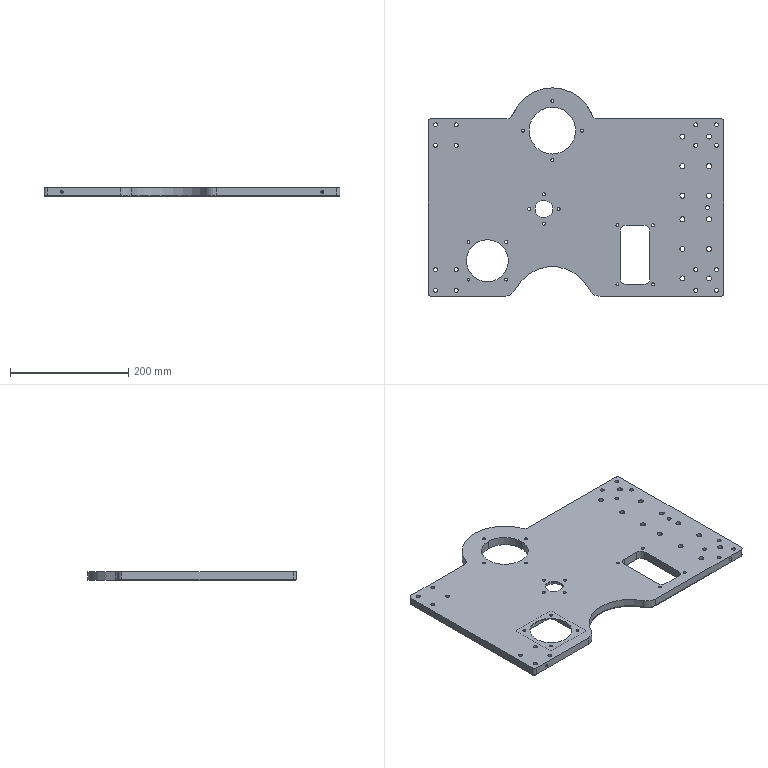NC program | Mastercam | posted with a generic post
Lines 2247 to 4160 of 11903, first 1756 of 1914 lines:
N2600 T4 M6
N2610 G0 G90 G17 G54 X-184.625 Y155.4 A0. S6000 M3
N2620 G43 H4 Z50. M8
N2630 Z1.3
N2640 G1 Z0. F600.
N2650 Y155.8 F3000.
N2660 G3 X-185.025 Y156.2 I-.4 J0.
N2670 G1 X-189.95
N2680 Y151.509
N2690 G3 X-189.55 Y151.109 I.4 J0.
N2700 G1 X-189.15
N2710 X-184.625 Y155.4
N2720 Z-.3 F600.
N2730 Y155.8 F3000.
N2740 G3 X-185.025 Y156.2 I-.4 J0.
N2750 G1 X-189.95
N2760 Y151.509
N2770 G3 X-189.55 Y151.109 I.4 J0.
N2780 G1 X-189.15
N2790 X-184.625 Y155.4
N2800 Z-.6 F600.
N2810 Y155.8 F3000.
N2820 G3 X-185.025 Y156.2 I-.4 J0.
N2830 G1 X-189.95
N2840 Y151.509
N2850 G3 X-189.55 Y151.109 I.4 J0.
N2860 G1 X-189.15
N2870 X-184.625 Y155.4
N2880 Z-.9 F600.
N2890 Y155.8 F3000.
N2900 G3 X-185.025 Y156.2 I-.4 J0.
N2910 G1 X-189.95
N2920 Y151.509
N2930 G3 X-189.55 Y151.109 I.4 J0.
N2940 G1 X-189.15
N2950 X-184.625 Y155.4
N2960 Z-1.2 F600.
N2970 Y155.8 F3000.
N2980 G3 X-185.025 Y156.2 I-.4 J0.
N2990 G1 X-189.95
N3000 Y151.509
N3010 G3 X-189.55 Y151.109 I.4 J0.
N3020 G1 X-189.15
N3030 X-184.625 Y155.4
N3040 Z-1.5 F600.
N3050 Y155.8 F3000.
N3060 G3 X-185.025 Y156.2 I-.4 J0.
N3070 G1 X-189.95
N3080 Y151.509
N3090 G3 X-189.55 Y151.109 I.4 J0.
N3100 G1 X-189.15
N3110 X-184.625 Y155.4
N3120 Z-1.8 F600.
N3130 Y155.8 F3000.
N3140 G3 X-185.025 Y156.2 I-.4 J0.
N3150 G1 X-189.95
N3160 Y151.509
N3170 G3 X-189.55 Y151.109 I.4 J0.
N3180 G1 X-189.15
N3190 X-184.625 Y155.4
N3200 Z-2.1 F600.
N3210 Y155.8 F3000.
N3220 G3 X-185.025 Y156.2 I-.4 J0.
N3230 G1 X-189.95
N3240 Y151.509
N3250 G3 X-189.55 Y151.109 I.4 J0.
N3260 G1 X-189.15
N3270 X-184.625 Y155.4
N3280 Z-2.4 F600.
N3290 Y155.8 F3000.
N3300 G3 X-185.025 Y156.2 I-.4 J0.
N3310 G1 X-189.95
N3320 Y151.509
N3330 G3 X-189.55 Y151.109 I.4 J0.
N3340 G1 X-189.15
N3350 X-184.625 Y155.4
N3360 Z-2.7 F600.
N3370 Y155.8 F3000.
N3380 G3 X-185.025 Y156.2 I-.4 J0.
N3390 G1 X-189.95
N3400 Y151.509
N3410 G3 X-189.55 Y151.109 I.4 J0.
N3420 G1 X-189.15
N3430 X-184.625 Y155.4
N3440 Z-3. F600.
N3450 Y155.8 F3000.
N3460 G3 X-185.025 Y156.2 I-.4 J0.
N3470 G1 X-189.95
N3480 Y151.509
N3490 G3 X-189.55 Y151.109 I.4 J0.
N3500 G1 X-189.15
N3510 X-184.625 Y155.4
N3520 Z-3.3 F600.
N3530 Y155.8 F3000.
N3540 G3 X-185.025 Y156.2 I-.4 J0.
N3550 G1 X-189.95
N3560 Y151.509
N3570 G3 X-189.55 Y151.109 I.4 J0.
N3580 G1 X-189.15
N3590 X-184.625 Y155.4
N3600 Z-3.6 F600.
N3610 Y155.8 F3000.
N3620 G3 X-185.025 Y156.2 I-.4 J0.
N3630 G1 X-189.95
N3640 Y151.509
N3650 G3 X-189.55 Y151.109 I.4 J0.
N3660 G1 X-189.15
N3670 X-184.625 Y155.4
N3680 Z-3.9 F600.
N3690 Y155.8 F3000.
N3700 G3 X-185.025 Y156.2 I-.4 J0.
N3710 G1 X-189.95
N3720 Y151.509
N3730 G3 X-189.55 Y151.109 I.4 J0.
N3740 G1 X-189.15
N3750 X-184.625 Y155.4
N3760 Z-4.2 F600.
N3770 Y155.8 F3000.
N3780 G3 X-185.025 Y156.2 I-.4 J0.
N3790 G1 X-189.95
N3800 Y151.509
N3810 G3 X-189.55 Y151.109 I.4 J0.
N3820 G1 X-189.15
N3830 X-184.625 Y155.4
N3840 Z-4.5 F600.
N3850 Y155.8 F3000.
N3860 G3 X-185.025 Y156.2 I-.4 J0.
N3870 G1 X-189.95
N3880 Y151.509
N3890 G3 X-189.55 Y151.109 I.4 J0.
N3900 G1 X-189.15
N3910 X-184.625 Y155.4
N3920 Z-4.8 F600.
N3930 Y155.8 F3000.
N3940 G3 X-185.025 Y156.2 I-.4 J0.
N3950 G1 X-189.95
N3960 Y151.509
N3970 G3 X-189.55 Y151.109 I.4 J0.
N3980 G1 X-189.15
N3990 X-184.625 Y155.4
N4000 Z-5.1 F600.
N4010 Y155.8 F3000.
N4020 G3 X-185.025 Y156.2 I-.4 J0.
N4030 G1 X-189.95
N4040 Y151.509
N4050 G3 X-189.55 Y151.109 I.4 J0.
N4060 G1 X-189.15
N4070 X-184.625 Y155.4
N4080 Z-5.4 F600.
N4090 Y155.8 F3000.
N4100 G3 X-185.025 Y156.2 I-.4 J0.
N4110 G1 X-189.95
N4120 Y151.509
N4130 G3 X-189.55 Y151.109 I.4 J0.
N4140 G1 X-189.15
N4150 X-184.625 Y155.4
N4160 Z-5.7 F600.
N4170 Y155.8 F3000.
N4180 G3 X-185.025 Y156.2 I-.4 J0.
N4190 G1 X-189.95
N4200 Y151.509
N4210 G3 X-189.55 Y151.109 I.4 J0.
N4220 G1 X-189.15
N4230 X-184.625 Y155.4
N4240 Z-6. F600.
N4250 Y155.8 F3000.
N4260 G3 X-185.025 Y156.2 I-.4 J0.
N4270 G1 X-189.95
N4280 Y151.509
N4290 G3 X-189.55 Y151.109 I.4 J0.
N4300 G1 X-189.15
N4310 X-184.625 Y155.4
N4320 Z-6.3 F600.
N4330 Y155.8 F3000.
N4340 G3 X-185.025 Y156.2 I-.4 J0.
N4350 G1 X-189.95
N4360 Y151.509
N4370 G3 X-189.55 Y151.109 I.4 J0.
N4380 G1 X-189.15
N4390 X-184.625 Y155.4
N4400 Z-6.6 F600.
N4410 Y155.8 F3000.
N4420 G3 X-185.025 Y156.2 I-.4 J0.
N4430 G1 X-189.95
N4440 Y151.509
N4450 G3 X-189.55 Y151.109 I.4 J0.
N4460 G1 X-189.15
N4470 X-184.625 Y155.4
N4480 Z-6.9 F600.
N4490 Y155.8 F3000.
N4500 G3 X-185.025 Y156.2 I-.4 J0.
N4510 G1 X-189.95
N4520 Y151.509
N4530 G3 X-189.55 Y151.109 I.4 J0.
N4540 G1 X-189.15
N4550 X-184.625 Y155.4
N4560 Z-7.2 F600.
N4570 Y155.8 F3000.
N4580 G3 X-185.025 Y156.2 I-.4 J0.
N4590 G1 X-189.95
N4600 Y151.509
N4610 G3 X-189.55 Y151.109 I.4 J0.
N4620 G1 X-189.15
N4630 X-184.625 Y155.4
N4640 Z-7.5 F600.
N4650 Y155.8 F3000.
N4660 G3 X-185.025 Y156.2 I-.4 J0.
N4670 G1 X-189.95
N4680 Y151.509
N4690 G3 X-189.55 Y151.109 I.4 J0.
N4700 G1 X-189.15
N4710 X-184.625 Y155.4
N4720 Z-7.8 F600.
N4730 Y155.8 F3000.
N4740 G3 X-185.025 Y156.2 I-.4 J0.
N4750 G1 X-189.95
N4760 Y151.509
N4770 G3 X-189.55 Y151.109 I.4 J0.
N4780 G1 X-189.15
N4790 X-184.625 Y155.4
N4800 Z-8.1 F600.
N4810 Y155.8 F3000.
N4820 G3 X-185.025 Y156.2 I-.4 J0.
N4830 G1 X-189.95
N4840 Y151.509
N4850 G3 X-189.55 Y151.109 I.4 J0.
N4860 G1 X-189.15
N4870 X-184.625 Y155.4
N4880 Z-8.4 F600.
N4890 Y155.8 F3000.
N4900 G3 X-185.025 Y156.2 I-.4 J0.
N4910 G1 X-189.95
N4920 Y151.509
N4930 G3 X-189.55 Y151.109 I.4 J0.
N4940 G1 X-189.15
N4950 X-184.625 Y155.4
N4960 Z-8.7 F600.
N4970 Y155.8 F3000.
N4980 G3 X-185.025 Y156.2 I-.4 J0.
N4990 G1 X-189.95
N5000 Y151.509
N5010 G3 X-189.55 Y151.109 I.4 J0.
N5020 G1 X-189.15
N5030 X-184.625 Y155.4
N5040 Z-9. F600.
N5050 Y155.8 F3000.
N5060 G3 X-185.025 Y156.2 I-.4 J0.
N5070 G1 X-189.95
N5080 Y151.509
N5090 G3 X-189.55 Y151.109 I.4 J0.
N5100 G1 X-189.15
N5110 X-184.625 Y155.4
N5120 Z-9.3 F600.
N5130 Y155.8 F3000.
N5140 G3 X-185.025 Y156.2 I-.4 J0.
N5150 G1 X-189.95
N5160 Y151.509
N5170 G3 X-189.55 Y151.109 I.4 J0.
N5180 G1 X-189.15
N5190 X-184.625 Y155.4
N5200 Z-9.6 F600.
N5210 Y155.8 F3000.
N5220 G3 X-185.025 Y156.2 I-.4 J0.
N5230 G1 X-189.95
N5240 Y151.509
N5250 G3 X-189.55 Y151.109 I.4 J0.
N5260 G1 X-189.15
N5270 X-184.625 Y155.4
N5280 Z-9.9 F600.
N5290 Y155.8 F3000.
N5300 G3 X-185.025 Y156.2 I-.4 J0.
N5310 G1 X-189.95
N5320 Y151.509
N5330 G3 X-189.55 Y151.109 I.4 J0.
N5340 G1 X-189.15
N5350 X-184.625 Y155.4
N5360 Z-10.2 F600.
N5370 Y155.8 F3000.
N5380 G3 X-185.025 Y156.2 I-.4 J0.
N5390 G1 X-189.95
N5400 Y151.509
N5410 G3 X-189.55 Y151.109 I.4 J0.
N5420 G1 X-189.15
N5430 X-184.625 Y155.4
N5440 Z-10.5 F600.
N5450 Y155.8 F3000.
N5460 G3 X-185.025 Y156.2 I-.4 J0.
N5470 G1 X-189.95
N5480 Y151.509
N5490 G3 X-189.55 Y151.109 I.4 J0.
N5500 G1 X-189.15
N5510 X-184.625 Y155.4
N5520 Z-10.8 F600.
N5530 Y155.8 F3000.
N5540 G3 X-185.025 Y156.2 I-.4 J0.
N5550 G1 X-189.95
N5560 Y151.509
N5570 G3 X-189.55 Y151.109 I.4 J0.
N5580 G1 X-189.15
N5590 X-184.625 Y155.4
N5600 Z-11.1 F600.
N5610 Y155.8 F3000.
N5620 G3 X-185.025 Y156.2 I-.4 J0.
N5630 G1 X-189.95
N5640 Y151.509
N5650 G3 X-189.55 Y151.109 I.4 J0.
N5660 G1 X-189.15
N5670 X-184.625 Y155.4
N5680 Z-11.4 F600.
N5690 Y155.8 F3000.
N5700 G3 X-185.025 Y156.2 I-.4 J0.
N5710 G1 X-189.95
N5720 Y151.509
N5730 G3 X-189.55 Y151.109 I.4 J0.
N5740 G1 X-189.15
N5750 X-184.625 Y155.4
N5760 Z-11.7 F600.
N5770 Y155.8 F3000.
N5780 G3 X-185.025 Y156.2 I-.4 J0.
N5790 G1 X-189.95
N5800 Y151.509
N5810 G3 X-189.55 Y151.109 I.4 J0.
N5820 G1 X-189.15
N5830 X-184.625 Y155.4
N5840 Z-12. F600.
N5850 Y155.8 F3000.
N5860 G3 X-185.025 Y156.2 I-.4 J0.
N5870 G1 X-189.95
N5880 Y151.509
N5890 G3 X-189.55 Y151.109 I.4 J0.
N5900 G1 X-189.15
N5910 X-184.625 Y155.4
N5920 Z-12.3 F600.
N5930 Y155.8 F3000.
N5940 G3 X-185.025 Y156.2 I-.4 J0.
N5950 G1 X-189.95
N5960 Y151.509
N5970 G3 X-189.55 Y151.109 I.4 J0.
N5980 G1 X-189.15
N5990 X-184.625 Y155.4
N6000 Z-12.6 F600.
N6010 Y155.8 F3000.
N6020 G3 X-185.025 Y156.2 I-.4 J0.
N6030 G1 X-189.95
N6040 Y151.509
N6050 G3 X-189.55 Y151.109 I.4 J0.
N6060 G1 X-189.15
N6070 X-184.625 Y155.4
N6080 Z-12.9 F600.
N6090 Y155.8 F3000.
N6100 G3 X-185.025 Y156.2 I-.4 J0.
N6110 G1 X-189.95
N6120 Y151.509
N6130 G3 X-189.55 Y151.109 I.4 J0.
N6140 G1 X-189.15
N6150 X-184.625 Y155.4
N6160 Z-13.2 F600.
N6170 Y155.8 F3000.
N6180 G3 X-185.025 Y156.2 I-.4 J0.
N6190 G1 X-189.95
N6200 Y151.509
N6210 G3 X-189.55 Y151.109 I.4 J0.
N6220 G1 X-189.15
N6230 X-184.625 Y155.4
N6240 Z-13.5 F600.
N6250 Y155.8 F3000.
N6260 G3 X-185.025 Y156.2 I-.4 J0.
N6270 G1 X-189.95
N6280 Y151.509
N6290 G3 X-189.55 Y151.109 I.4 J0.
N6300 G1 X-189.15
N6310 X-184.625 Y155.4
N6320 Z-13.8 F600.
N6330 Y155.8 F3000.
N6340 G3 X-185.025 Y156.2 I-.4 J0.
N6350 G1 X-189.95
N6360 Y151.509
N6370 G3 X-189.55 Y151.109 I.4 J0.
N6380 G1 X-189.15
N6390 G0 Z50.
N6400 Y81.2
N6410 Z1.3
N6420 G1 Z0. F600.
N6430 X-189.55 F3000.
N6440 G3 X-189.95 Y80.8 I0. J-.4
N6450 G1 Y76.3
N6460 X-185.2
N6470 G3 X-184.8 Y76.7 I0. J.4
N6480 G1 Y77.1
N6490 X-189.15 Y81.2
N6500 Z-.3 F600.
N6510 X-189.55 F3000.
N6520 G3 X-189.95 Y80.8 I0. J-.4
N6530 G1 Y76.3
N6540 X-185.2
N6550 G3 X-184.8 Y76.7 I0. J.4
N6560 G1 Y77.1
N6570 X-189.15 Y81.2
N6580 Z-.6 F600.
N6590 X-189.55 F3000.
N6600 G3 X-189.95 Y80.8 I0. J-.4
N6610 G1 Y76.3
N6620 X-185.2
N6630 G3 X-184.8 Y76.7 I0. J.4
N6640 G1 Y77.1
N6650 X-189.15 Y81.2
N6660 Z-.9 F600.
N6670 X-189.55 F3000.
N6680 G3 X-189.95 Y80.8 I0. J-.4
N6690 G1 Y76.3
N6700 X-185.2
N6710 G3 X-184.8 Y76.7 I0. J.4
N6720 G1 Y77.1
N6730 X-189.15 Y81.2
N6740 Z-1.2 F600.
N6750 X-189.55 F3000.
N6760 G3 X-189.95 Y80.8 I0. J-.4
N6770 G1 Y76.3
N6780 X-185.2
N6790 G3 X-184.8 Y76.7 I0. J.4
N6800 G1 Y77.1
N6810 X-189.15 Y81.2
N6820 Z-1.5 F600.
N6830 X-189.55 F3000.
N6840 G3 X-189.95 Y80.8 I0. J-.4
N6850 G1 Y76.3
N6860 X-185.2
N6870 G3 X-184.8 Y76.7 I0. J.4
N6880 G1 Y77.1
N6890 X-189.15 Y81.2
N6900 Z-1.8 F600.
N6910 X-189.55 F3000.
N6920 G3 X-189.95 Y80.8 I0. J-.4
N6930 G1 Y76.3
N6940 X-185.2
N6950 G3 X-184.8 Y76.7 I0. J.4
N6960 G1 Y77.1
N6970 X-189.15 Y81.2
N6980 Z-2.1 F600.
N6990 X-189.55 F3000.
N7000 G3 X-189.95 Y80.8 I0. J-.4
N7010 G1 Y76.3
N7020 X-185.2
N7030 G3 X-184.8 Y76.7 I0. J.4
N7040 G1 Y77.1
N7050 X-189.15 Y81.2
N7060 Z-2.4 F600.
N7070 X-189.55 F3000.
N7080 G3 X-189.95 Y80.8 I0. J-.4
N7090 G1 Y76.3
N7100 X-185.2
N7110 G3 X-184.8 Y76.7 I0. J.4
N7120 G1 Y77.1
N7130 X-189.15 Y81.2
N7140 Z-2.7 F600.
N7150 X-189.55 F3000.
N7160 G3 X-189.95 Y80.8 I0. J-.4
N7170 G1 Y76.3
N7180 X-185.2
N7190 G3 X-184.8 Y76.7 I0. J.4
N7200 G1 Y77.1
N7210 X-189.15 Y81.2
N7220 Z-3. F600.
N7230 X-189.55 F3000.
N7240 G3 X-189.95 Y80.8 I0. J-.4
N7250 G1 Y76.3
N7260 X-185.2
N7270 G3 X-184.8 Y76.7 I0. J.4
N7280 G1 Y77.1
N7290 X-189.15 Y81.2
N7300 Z-3.3 F600.
N7310 X-189.55 F3000.
N7320 G3 X-189.95 Y80.8 I0. J-.4
N7330 G1 Y76.3
N7340 X-185.2
N7350 G3 X-184.8 Y76.7 I0. J.4
N7360 G1 Y77.1
N7370 X-189.15 Y81.2
N7380 Z-3.6 F600.
N7390 X-189.55 F3000.
N7400 G3 X-189.95 Y80.8 I0. J-.4
N7410 G1 Y76.3
N7420 X-185.2
N7430 G3 X-184.8 Y76.7 I0. J.4
N7440 G1 Y77.1
N7450 X-189.15 Y81.2
N7460 Z-3.9 F600.
N7470 X-189.55 F3000.
N7480 G3 X-189.95 Y80.8 I0. J-.4
N7490 G1 Y76.3
N7500 X-185.2
N7510 G3 X-184.8 Y76.7 I0. J.4
N7520 G1 Y77.1
N7530 X-189.15 Y81.2
N7540 Z-4.2 F600.
N7550 X-189.55 F3000.
N7560 G3 X-189.95 Y80.8 I0. J-.4
N7570 G1 Y76.3
N7580 X-185.2
N7590 G3 X-184.8 Y76.7 I0. J.4
N7600 G1 Y77.1
N7610 X-189.15 Y81.2
N7620 Z-4.5 F600.
N7630 X-189.55 F3000.
N7640 G3 X-189.95 Y80.8 I0. J-.4
N7650 G1 Y76.3
N7660 X-185.2
N7670 G3 X-184.8 Y76.7 I0. J.4
N7680 G1 Y77.1
N7690 X-189.15 Y81.2
N7700 Z-4.8 F600.
N7710 X-189.55 F3000.
N7720 G3 X-189.95 Y80.8 I0. J-.4
N7730 G1 Y76.3
N7740 X-185.2
N7750 G3 X-184.8 Y76.7 I0. J.4
N7760 G1 Y77.1
N7770 X-189.15 Y81.2
N7780 Z-5.1 F600.
N7790 X-189.55 F3000.
N7800 G3 X-189.95 Y80.8 I0. J-.4
N7810 G1 Y76.3
N7820 X-185.2
N7830 G3 X-184.8 Y76.7 I0. J.4
N7840 G1 Y77.1
N7850 X-189.15 Y81.2
N7860 Z-5.4 F600.
N7870 X-189.55 F3000.
N7880 G3 X-189.95 Y80.8 I0. J-.4
N7890 G1 Y76.3
N7900 X-185.2
N7910 G3 X-184.8 Y76.7 I0. J.4
N7920 G1 Y77.1
N7930 X-189.15 Y81.2
N7940 Z-5.7 F600.
N7950 X-189.55 F3000.
N7960 G3 X-189.95 Y80.8 I0. J-.4
N7970 G1 Y76.3
N7980 X-185.2
N7990 G3 X-184.8 Y76.7 I0. J.4
N8000 G1 Y77.1
N8010 X-189.15 Y81.2
N8020 Z-6. F600.
N8030 X-189.55 F3000.
N8040 G3 X-189.95 Y80.8 I0. J-.4
N8050 G1 Y76.3
N8060 X-185.2
N8070 G3 X-184.8 Y76.7 I0. J.4
N8080 G1 Y77.1
N8090 X-189.15 Y81.2
N8100 Z-6.3 F600.
N8110 X-189.55 F3000.
N8120 G3 X-189.95 Y80.8 I0. J-.4
N8130 G1 Y76.3
N8140 X-185.2
N8150 G3 X-184.8 Y76.7 I0. J.4
N8160 G1 Y77.1
N8170 X-189.15 Y81.2
N8180 Z-6.6 F600.
N8190 X-189.55 F3000.
N8200 G3 X-189.95 Y80.8 I0. J-.4
N8210 G1 Y76.3
N8220 X-185.2
N8230 G3 X-184.8 Y76.7 I0. J.4
N8240 G1 Y77.1
N8250 X-189.15 Y81.2
N8260 Z-6.9 F600.
N8270 X-189.55 F3000.
N8280 G3 X-189.95 Y80.8 I0. J-.4
N8290 G1 Y76.3
N8300 X-185.2
N8310 G3 X-184.8 Y76.7 I0. J.4
N8320 G1 Y77.1
N8330 X-189.15 Y81.2
N8340 Z-7.2 F600.
N8350 X-189.55 F3000.
N8360 G3 X-189.95 Y80.8 I0. J-.4
N8370 G1 Y76.3
N8380 X-185.2
N8390 G3 X-184.8 Y76.7 I0. J.4
N8400 G1 Y77.1
N8410 X-189.15 Y81.2
N8420 Z-7.5 F600.
N8430 X-189.55 F3000.
N8440 G3 X-189.95 Y80.8 I0. J-.4
N8450 G1 Y76.3
N8460 X-185.2
N8470 G3 X-184.8 Y76.7 I0. J.4
N8480 G1 Y77.1
N8490 X-189.15 Y81.2
N8500 Z-7.8 F600.
N8510 X-189.55 F3000.
N8520 G3 X-189.95 Y80.8 I0. J-.4
N8530 G1 Y76.3
N8540 X-185.2
N8550 G3 X-184.8 Y76.7 I0. J.4
N8560 G1 Y77.1
N8570 X-189.15 Y81.2
N8580 Z-8.1 F600.
N8590 X-189.55 F3000.
N8600 G3 X-189.95 Y80.8 I0. J-.4
N8610 G1 Y76.3
N8620 X-185.2
N8630 G3 X-184.8 Y76.7 I0. J.4
N8640 G1 Y77.1
N8650 X-189.15 Y81.2
N8660 Z-8.4 F600.
N8670 X-189.55 F3000.
N8680 G3 X-189.95 Y80.8 I0. J-.4
N8690 G1 Y76.3
N8700 X-185.2
N8710 G3 X-184.8 Y76.7 I0. J.4
N8720 G1 Y77.1
N8730 X-189.15 Y81.2
N8740 Z-8.7 F600.
N8750 X-189.55 F3000.
N8760 G3 X-189.95 Y80.8 I0. J-.4
N8770 G1 Y76.3
N8780 X-185.2
N8790 G3 X-184.8 Y76.7 I0. J.4
N8800 G1 Y77.1
N8810 X-189.15 Y81.2
N8820 Z-9. F600.
N8830 X-189.55 F3000.
N8840 G3 X-189.95 Y80.8 I0. J-.4
N8850 G1 Y76.3
N8860 X-185.2
N8870 G3 X-184.8 Y76.7 I0. J.4
N8880 G1 Y77.1
N8890 X-189.15 Y81.2
N8900 Z-9.3 F600.
N8910 X-189.55 F3000.
N8920 G3 X-189.95 Y80.8 I0. J-.4
N8930 G1 Y76.3
N8940 X-185.2
N8950 G3 X-184.8 Y76.7 I0. J.4
N8960 G1 Y77.1
N8970 X-189.15 Y81.2
N8980 Z-9.6 F600.
N8990 X-189.55 F3000.
N9000 G3 X-189.95 Y80.8 I0. J-.4
N9010 G1 Y76.3
N9020 X-185.2
N9030 G3 X-184.8 Y76.7 I0. J.4
N9040 G1 Y77.1
N9050 X-189.15 Y81.2
N9060 Z-9.9 F600.
N9070 X-189.55 F3000.
N9080 G3 X-189.95 Y80.8 I0. J-.4
N9090 G1 Y76.3
N9100 X-185.2
N9110 G3 X-184.8 Y76.7 I0. J.4
N9120 G1 Y77.1
N9130 X-189.15 Y81.2
N9140 Z-10.2 F600.
N9150 X-189.55 F3000.
N9160 G3 X-189.95 Y80.8 I0. J-.4
N9170 G1 Y76.3
N9180 X-185.2
N9190 G3 X-184.8 Y76.7 I0. J.4
N9200 G1 Y77.1
N9210 X-189.15 Y81.2
N9220 Z-10.5 F600.
N9230 X-189.55 F3000.
N9240 G3 X-189.95 Y80.8 I0. J-.4
N9250 G1 Y76.3
N9260 X-185.2
N9270 G3 X-184.8 Y76.7 I0. J.4
N9280 G1 Y77.1
N9290 X-189.15 Y81.2
N9300 Z-10.8 F600.
N9310 X-189.55 F3000.
N9320 G3 X-189.95 Y80.8 I0. J-.4
N9330 G1 Y76.3
N9340 X-185.2
N9350 G3 X-184.8 Y76.7 I0. J.4
N9360 G1 Y77.1
N9370 X-189.15 Y81.2
N9380 Z-11.1 F600.
N9390 X-189.55 F3000.
N9400 G3 X-189.95 Y80.8 I0. J-.4
N9410 G1 Y76.3
N9420 X-185.2
N9430 G3 X-184.8 Y76.7 I0. J.4
N9440 G1 Y77.1
N9450 X-189.15 Y81.2
N9460 Z-11.4 F600.
N9470 X-189.55 F3000.
N9480 G3 X-189.95 Y80.8 I0. J-.4
N9490 G1 Y76.3
N9500 X-185.2
N9510 G3 X-184.8 Y76.7 I0. J.4
N9520 G1 Y77.1
N9530 X-189.15 Y81.2
N9540 Z-11.7 F600.
N9550 X-189.55 F3000.
N9560 G3 X-189.95 Y80.8 I0. J-.4
N9570 G1 Y76.3
N9580 X-185.2
N9590 G3 X-184.8 Y76.7 I0. J.4
N9600 G1 Y77.1
N9610 X-189.15 Y81.2
N9620 Z-12. F600.
N9630 X-189.55 F3000.
N9640 G3 X-189.95 Y80.8 I0. J-.4
N9650 G1 Y76.3
N9660 X-185.2
N9670 G3 X-184.8 Y76.7 I0. J.4
N9680 G1 Y77.1
N9690 X-189.15 Y81.2
N9700 Z-12.3 F600.
N9710 X-189.55 F3000.
N9720 G3 X-189.95 Y80.8 I0. J-.4
N9730 G1 Y76.3
N9740 X-185.2
N9750 G3 X-184.8 Y76.7 I0. J.4
N9760 G1 Y77.1
N9770 X-189.15 Y81.2
N9780 Z-12.6 F600.
N9790 X-189.55 F3000.
N9800 G3 X-189.95 Y80.8 I0. J-.4
N9810 G1 Y76.3
N9820 X-185.2
N9830 G3 X-184.8 Y76.7 I0. J.4
N9840 G1 Y77.1
N9850 X-189.15 Y81.2
N9860 Z-12.9 F600.
N9870 X-189.55 F3000.
N9880 G3 X-189.95 Y80.8 I0. J-.4
N9890 G1 Y76.3
N9900 X-185.2
N9910 G3 X-184.8 Y76.7 I0. J.4
N9920 G1 Y77.1
N9930 X-189.15 Y81.2
N9940 Z-13.2 F600.
N9950 X-189.55 F3000.
N9960 G3 X-189.95 Y80.8 I0. J-.4
N9970 G1 Y76.3
N9980 X-185.2
N9990 G3 X-184.8 Y76.7 I0. J.4
N100 G1 Y77.1
N110 X-189.15 Y81.2
N120 Z-13.5 F600.
N130 X-189.55 F3000.
N140 G3 X-189.95 Y80.8 I0. J-.4
N150 G1 Y76.3
N160 X-185.2
N170 G3 X-184.8 Y76.7 I0. J.4
N180 G1 Y77.1
N190 X-189.15 Y81.2
N200 Z-13.8 F600.
N210 X-189.55 F3000.
N220 G3 X-189.95 Y80.8 I0. J-.4
N230 G1 Y76.3
N240 X-185.2
N250 G3 X-184.8 Y76.7 I0. J.4
N260 G1 Y77.1
N270 G0 Z50.
N280 X-115.2
N290 Z1.3
N300 G1 Z0. F600.
N310 Y76.7 F3000.
N320 G3 X-114.8 Y76.3 I.4 J0.
N330 G1 X-110.05
N340 Y80.882
N350 G3 X-110.45 Y81.282 I-.4 J0.
N360 G1 X-110.85
N370 X-115.2 Y77.1
N380 Z-.3 F600.
N390 Y76.7 F3000.
N400 G3 X-114.8 Y76.3 I.4 J0.
N410 G1 X-110.05
N420 Y80.882
N430 G3 X-110.45 Y81.282 I-.4 J0.
N440 G1 X-110.85
N450 X-115.2 Y77.1
N460 Z-.6 F600.
N470 Y76.7 F3000.
N480 G3 X-114.8 Y76.3 I.4 J0.
N490 G1 X-110.05
N500 Y80.882
N510 G3 X-110.45 Y81.282 I-.4 J0.
N520 G1 X-110.85
N530 X-115.2 Y77.1
N540 Z-.9 F600.
N550 Y76.7 F3000.
N560 G3 X-114.8 Y76.3 I.4 J0.
N570 G1 X-110.05
N580 Y80.882
N590 G3 X-110.45 Y81.282 I-.4 J0.
N600 G1 X-110.85
N610 X-115.2 Y77.1
N620 Z-1.2 F600.
N630 Y76.7 F3000.
N640 G3 X-114.8 Y76.3 I.4 J0.
N650 G1 X-110.05
N660 Y80.882
N670 G3 X-110.45 Y81.282 I-.4 J0.
N680 G1 X-110.85
N690 X-115.2 Y77.1
N700 Z-1.5 F600.
N710 Y76.7 F3000.
N720 G3 X-114.8 Y76.3 I.4 J0.
N730 G1 X-110.05
N740 Y80.882
N750 G3 X-110.45 Y81.282 I-.4 J0.
N760 G1 X-110.85
N770 X-115.2 Y77.1
N780 Z-1.8 F600.
N790 Y76.7 F3000.
N800 G3 X-114.8 Y76.3 I.4 J0.
N810 G1 X-110.05
N820 Y80.882
N830 G3 X-110.45 Y81.282 I-.4 J0.
N840 G1 X-110.85
N850 X-115.2 Y77.1
N860 Z-2.1 F600.
N870 Y76.7 F3000.
N880 G3 X-114.8 Y76.3 I.4 J0.
N890 G1 X-110.05
N900 Y80.882
N910 G3 X-110.45 Y81.282 I-.4 J0.
N920 G1 X-110.85
N930 X-115.2 Y77.1
N940 Z-2.4 F600.
N950 Y76.7 F3000.
N960 G3 X-114.8 Y76.3 I.4 J0.
N970 G1 X-110.05
N980 Y80.882
N990 G3 X-110.45 Y81.282 I-.4 J0.
N1000 G1 X-110.85
N1010 X-115.2 Y77.1
N1020 Z-2.7 F600.
N1030 Y76.7 F3000.
N1040 G3 X-114.8 Y76.3 I.4 J0.
N1050 G1 X-110.05
N1060 Y80.882
N1070 G3 X-110.45 Y81.282 I-.4 J0.
N1080 G1 X-110.85
N1090 X-115.2 Y77.1
N1100 Z-3. F600.
N1110 Y76.7 F3000.
N1120 G3 X-114.8 Y76.3 I.4 J0.
N1130 G1 X-110.05
N1140 Y80.882
N1150 G3 X-110.45 Y81.282 I-.4 J0.
N1160 G1 X-110.85
N1170 X-115.2 Y77.1
N1180 Z-3.3 F600.
N1190 Y76.7 F3000.
N1200 G3 X-114.8 Y76.3 I.4 J0.
N1210 G1 X-110.05
N1220 Y80.882
N1230 G3 X-110.45 Y81.282 I-.4 J0.
N1240 G1 X-110.85
N1250 X-115.2 Y77.1
N1260 Z-3.6 F600.
N1270 Y76.7 F3000.
N1280 G3 X-114.8 Y76.3 I.4 J0.
N1290 G1 X-110.05
N1300 Y80.882
N1310 G3 X-110.45 Y81.282 I-.4 J0.
N1320 G1 X-110.85
N1330 X-115.2 Y77.1
N1340 Z-3.9 F600.
N1350 Y76.7 F3000.
N1360 G3 X-114.8 Y76.3 I.4 J0.
N1370 G1 X-110.05
N1380 Y80.882
N1390 G3 X-110.45 Y81.282 I-.4 J0.
N1400 G1 X-110.85
N1410 X-115.2 Y77.1
N1420 Z-4.2 F600.
N1430 Y76.7 F3000.
N1440 G3 X-114.8 Y76.3 I.4 J0.
N1450 G1 X-110.05
N1460 Y80.882
N1470 G3 X-110.45 Y81.282 I-.4 J0.
N1480 G1 X-110.85
N1490 X-115.2 Y77.1
N1500 Z-4.5 F600.
N1510 Y76.7 F3000.
N1520 G3 X-114.8 Y76.3 I.4 J0.
N1530 G1 X-110.05
N1540 Y80.882
N1550 G3 X-110.45 Y81.282 I-.4 J0.
N1560 G1 X-110.85
N1570 X-115.2 Y77.1
N1580 Z-4.8 F600.
N1590 Y76.7 F3000.
N1600 G3 X-114.8 Y76.3 I.4 J0.
N1610 G1 X-110.05
N1620 Y80.882
N1630 G3 X-110.45 Y81.282 I-.4 J0.
N1640 G1 X-110.85
N1650 X-115.2 Y77.1
N1660 Z-5.1 F600.
N1670 Y76.7 F3000.
N1680 G3 X-114.8 Y76.3 I.4 J0.
N1690 G1 X-110.05
N1700 Y80.882
N1710 G3 X-110.45 Y81.282 I-.4 J0.
N1720 G1 X-110.85
N1730 X-115.2 Y77.1
N1740 Z-5.4 F600.
N1750 Y76.7 F3000.
N1760 G3 X-114.8 Y76.3 I.4 J0.
N1770 G1 X-110.05
N1780 Y80.882
N1790 G3 X-110.45 Y81.282 I-.4 J0.
N1800 G1 X-110.85
N1810 X-115.2 Y77.1
N1820 Z-5.7 F600.
N1830 Y76.7 F3000.
N1840 G3 X-114.8 Y76.3 I.4 J0.
N1850 G1 X-110.05
N1860 Y80.882
N1870 G3 X-110.45 Y81.282 I-.4 J0.
N1880 G1 X-110.85
N1890 X-115.2 Y77.1
N1900 Z-6. F600.
N1910 Y76.7 F3000.
N1920 G3 X-114.8 Y76.3 I.4 J0.
N1930 G1 X-110.05
N1940 Y80.882
N1950 G3 X-110.45 Y81.282 I-.4 J0.
N1960 G1 X-110.85
N1970 X-115.2 Y77.1
N1980 Z-6.3 F600.
N1990 Y76.7 F3000.
N2000 G3 X-114.8 Y76.3 I.4 J0.
N2010 G1 X-110.05
N2020 Y80.882
N2030 G3 X-110.45 Y81.282 I-.4 J0.
N2040 G1 X-110.85
N2050 X-115.2 Y77.1
N2060 Z-6.6 F600.
N2070 Y76.7 F3000.
N2080 G3 X-114.8 Y76.3 I.4 J0.
N2090 G1 X-110.05
N2100 Y80.882
N2110 G3 X-110.45 Y81.282 I-.4 J0.
N2120 G1 X-110.85
N2130 X-115.2 Y77.1
N2140 Z-6.9 F600.
N2150 Y76.7 F3000.
N2160 G3 X-114.8 Y76.3 I.4 J0.
N2170 G1 X-110.05
N2180 Y80.882
N2190 G3 X-110.45 Y81.282 I-.4 J0.
N2200 G1 X-110.85
N2210 X-115.2 Y77.1
N2220 Z-7.2 F600.
N2230 Y76.7 F3000.
N2240 G3 X-114.8 Y76.3 I.4 J0.
N2250 G1 X-110.05
N2260 Y80.882
N2270 G3 X-110.45 Y81.282 I-.4 J0.
N2280 G1 X-110.85
N2290 X-115.2 Y77.1
N2300 Z-7.5 F600.
N2310 Y76.7 F3000.
N2320 G3 X-114.8 Y76.3 I.4 J0.
N2330 G1 X-110.05
N2340 Y80.882
N2350 G3 X-110.45 Y81.282 I-.4 J0.
N2360 G1 X-110.85
N2370 X-115.2 Y77.1
N2380 Z-7.8 F600.
N2390 Y76.7 F3000.
N2400 G3 X-114.8 Y76.3 I.4 J0.
N2410 G1 X-110.05
N2420 Y80.882
N2430 G3 X-110.45 Y81.282 I-.4 J0.
N2440 G1 X-110.85
N2450 X-115.2 Y77.1
N2460 Z-8.1 F600.
N2470 Y76.7 F3000.
N2480 G3 X-114.8 Y76.3 I.4 J0.
N2490 G1 X-110.05
N2500 Y80.882
N2510 G3 X-110.45 Y81.282 I-.4 J0.
N2520 G1 X-110.85
N2530 X-115.2 Y77.1
N2540 Z-8.4 F600.
N2550 Y76.7 F3000.
N2560 G3 X-114.8 Y76.3 I.4 J0.
N2570 G1 X-110.05
N2580 Y80.882
N2590 G3 X-110.45 Y81.282 I-.4 J0.
N2600 G1 X-110.85
N2610 X-115.2 Y77.1
N2620 Z-8.7 F600.
N2630 Y76.7 F3000.
N2640 G3 X-114.8 Y76.3 I.4 J0.
N2650 G1 X-110.05
N2660 Y80.882
N2670 G3 X-110.45 Y81.282 I-.4 J0.
N2680 G1 X-110.85
N2690 X-115.2 Y77.1
N2700 Z-9. F600.
N2710 Y76.7 F3000.
N2720 G3 X-114.8 Y76.3 I.4 J0.
N2730 G1 X-110.05
N2740 Y80.882
N2750 G3 X-110.45 Y81.282 I-.4 J0.
N2760 G1 X-110.85
N2770 X-115.2 Y77.1
N2780 Z-9.3 F600.
N2790 Y76.7 F3000.
N2800 G3 X-114.8 Y76.3 I.4 J0.
N2810 G1 X-110.05
N2820 Y80.882
N2830 G3 X-110.45 Y81.282 I-.4 J0.
N2840 G1 X-110.85
N2850 X-115.2 Y77.1
N2860 Z-9.6 F600.
N2870 Y76.7 F3000.
N2880 G3 X-114.8 Y76.3 I.4 J0.
N2890 G1 X-110.05
N2900 Y80.882
N2910 G3 X-110.45 Y81.282 I-.4 J0.
N2920 G1 X-110.85
N2930 X-115.2 Y77.1
N2940 Z-9.9 F600.
N2950 Y76.7 F3000.
N2960 G3 X-114.8 Y76.3 I.4 J0.
N2970 G1 X-110.05
N2980 Y80.882
N2990 G3 X-110.45 Y81.282 I-.4 J0.
N3000 G1 X-110.85
N3010 X-115.2 Y77.1
N3020 Z-10.2 F600.
N3030 Y76.7 F3000.
N3040 G3 X-114.8 Y76.3 I.4 J0.
N3050 G1 X-110.05
N3060 Y80.882
N3070 G3 X-110.45 Y81.282 I-.4 J0.
N3080 G1 X-110.85
N3090 X-115.2 Y77.1
N3100 Z-10.5 F600.
N3110 Y76.7 F3000.
N3120 G3 X-114.8 Y76.3 I.4 J0.
N3130 G1 X-110.05
N3140 Y80.882
N3150 G3 X-110.45 Y81.282 I-.4 J0.
N3160 G1 X-110.85
N3170 X-115.2 Y77.1
N3180 Z-10.8 F600.
N3190 Y76.7 F3000.
N3200 G3 X-114.8 Y76.3 I.4 J0.
N3210 G1 X-110.05
N3220 Y80.882
N3230 G3 X-110.45 Y81.282 I-.4 J0.
N3240 G1 X-110.85
N3250 X-115.2 Y77.1
N3260 Z-11.1 F600.
N3270 Y76.7 F3000.
N3280 G3 X-114.8 Y76.3 I.4 J0.
N3290 G1 X-110.05
N3300 Y80.882
N3310 G3 X-110.45 Y81.282 I-.4 J0.
N3320 G1 X-110.85
N3330 X-115.2 Y77.1
N3340 Z-11.4 F600.
N3350 Y76.7 F3000.
N3360 G3 X-114.8 Y76.3 I.4 J0.
N3370 G1 X-110.05
N3380 Y80.882
N3390 G3 X-110.45 Y81.282 I-.4 J0.
N3400 G1 X-110.85
N3410 X-115.2 Y77.1
N3420 Z-11.7 F600.
N3430 Y76.7 F3000.
N3440 G3 X-114.8 Y76.3 I.4 J0.
N3450 G1 X-110.05
N3460 Y80.882
N3470 G3 X-110.45 Y81.282 I-.4 J0.
N3480 G1 X-110.85
N3490 X-115.2 Y77.1
N3500 Z-12. F600.
N3510 Y76.7 F3000.
N3520 G3 X-114.8 Y76.3 I.4 J0.
N3530 G1 X-110.05
N3540 Y80.882
N3550 G3 X-110.45 Y81.282 I-.4 J0.
N3560 G1 X-110.85
N3570 X-115.2 Y77.1
N3580 Z-12.3 F600.
N3590 Y76.7 F3000.
N3600 G3 X-114.8 Y76.3 I.4 J0.
N3610 G1 X-110.05
N3620 Y80.882
N3630 G3 X-110.45 Y81.282 I-.4 J0.
N3640 G1 X-110.85
N3650 X-115.2 Y77.1
N3660 Z-12.6 F600.
N3670 Y76.7 F3000.
N3680 G3 X-114.8 Y76.3 I.4 J0.
N3690 G1 X-110.05
N3700 Y80.882
N3710 G3 X-110.45 Y81.282 I-.4 J0.
N3720 G1 X-110.85
N3730 X-115.2 Y77.1
N3740 Z-12.9 F600.
N3750 Y76.7 F3000.
N3760 G3 X-114.8 Y76.3 I.4 J0.
N3770 G1 X-110.05
N3780 Y80.882
N3790 G3 X-110.45 Y81.282 I-.4 J0.
N3800 G1 X-110.85
N3810 X-115.2 Y77.1
N3820 Z-13.2 F600.
N3830 Y76.7 F3000.
N3840 G3 X-114.8 Y76.3 I.4 J0.
N3850 G1 X-110.05
N3860 Y80.882
N3870 G3 X-110.45 Y81.282 I-.4 J0.
N3880 G1 X-110.85
N3890 X-115.2 Y77.1
N3900 Z-13.5 F600.
N3910 Y76.7 F3000.
N3920 G3 X-114.8 Y76.3 I.4 J0.
N3930 G1 X-110.05
N3940 Y80.882
N3950 G3 X-110.45 Y81.282 I-.4 J0.
N3960 G1 X-110.85
N3970 X-115.2 Y77.1
N3980 Z-13.8 F600.
N3990 Y76.7 F3000.
N4000 G3 X-114.8 Y76.3 I.4 J0.
N4010 G1 X-110.05
N4020 Y80.882
N4030 G3 X-110.45 Y81.282 I-.4 J0.
N4040 G1 X-110.85
N4050 G0 Z50.
N4060 Y151.185
N4070 Z1.3
N4080 G1 Z0. F600.
N4090 X-110.45 F3000.
N4100 G3 X-110.05 Y151.585 I0. J.4
N4110 G1 Y156.2
N4120 X-115.015
N4130 G3 X-115.415 Y155.8 I0. J-.4
N4140 G1 Y155.4
N4150 X-110.85 Y151.185
N4160 Z-.3 F600.
N4170 X-110.45 F3000.
N4180 G3 X-110.05 Y151.585 I0. J.4
N4190 G1 Y156.2
N4200 X-115.015
N4210 G3 X-115.415 Y155.8 I0. J-.4
N4220 G1 Y155.4
N4230 X-110.85 Y151.185
N4240 Z-.6 F600.
N4250 X-110.45 F3000.
N4260 G3 X-110.05 Y151.585 I0. J.4
N4270 G1 Y156.2
N4280 X-115.015
N4290 G3 X-115.415 Y155.8 I0. J-.4
N4300 G1 Y155.4
N4310 X-110.85 Y151.185
N4320 Z-.9 F600.
N4330 X-110.45 F3000.
N4340 G3 X-110.05 Y151.585 I0. J.4
N4350 G1 Y156.2
N4360 X-115.015
N4370 G3 X-115.415 Y155.8 I0. J-.4
N4380 G1 Y155.4
N4390 X-110.85 Y151.185
N4400 Z-1.2 F600.
N4410 X-110.45 F3000.
N4420 G3 X-110.05 Y151.585 I0. J.4
N4430 G1 Y156.2
N4440 X-115.015
N4450 G3 X-115.415 Y155.8 I0. J-.4
N4460 G1 Y155.4
N4470 X-110.85 Y151.185
N4480 Z-1.5 F600.
N4490 X-110.45 F3000.
N4500 G3 X-110.05 Y151.585 I0. J.4
N4510 G1 Y156.2
N4520 X-115.015
N4530 G3 X-115.415 Y155.8 I0. J-.4
N4540 G1 Y155.4
N4550 X-110.85 Y151.185
N4560 Z-1.8 F600.
N4570 X-110.45 F3000.
N4580 G3 X-110.05 Y151.585 I0. J.4
N4590 G1 Y156.2
N4600 X-115.015
N4610 G3 X-115.415 Y155.8 I0. J-.4
N4620 G1 Y155.4
N4630 X-110.85 Y151.185
N4640 Z-2.1 F600.
N4650 X-110.45 F3000.
N4660 G3 X-110.05 Y151.585 I0. J.4
N4670 G1 Y156.2
N4680 X-115.015
N4690 G3 X-115.415 Y155.8 I0. J-.4
N4700 G1 Y155.4
N4710 X-110.85 Y151.185
N4720 Z-2.4 F600.
N4730 X-110.45 F3000.
N4740 G3 X-110.05 Y151.585 I0. J.4
N4750 G1 Y156.2
N4760 X-115.015
N4770 G3 X-115.415 Y155.8 I0. J-.4
N4780 G1 Y155.4
N4790 X-110.85 Y151.185
N4800 Z-2.7 F600.
N4810 X-110.45 F3000.
N4820 G3 X-110.05 Y151.585 I0. J.4
N4830 G1 Y156.2
N4840 X-115.015
N4850 G3 X-115.415 Y155.8 I0. J-.4
N4860 G1 Y155.4
N4870 X-110.85 Y151.185
N4880 Z-3. F600.
N4890 X-110.45 F3000.
N4900 G3 X-110.05 Y151.585 I0. J.4
N4910 G1 Y156.2
N4920 X-115.015
N4930 G3 X-115.415 Y155.8 I0. J-.4
N4940 G1 Y155.4
N4950 X-110.85 Y151.185
N4960 Z-3.3 F600.
N4970 X-110.45 F3000.
N4980 G3 X-110.05 Y151.585 I0. J.4
N4990 G1 Y156.2
N5000 X-115.015
N5010 G3 X-115.415 Y155.8 I0. J-.4
N5020 G1 Y155.4
N5030 X-110.85 Y151.185
N5040 Z-3.6 F600.
N5050 X-110.45 F3000.
N5060 G3 X-110.05 Y151.585 I0. J.4
N5070 G1 Y156.2
N5080 X-115.015
N5090 G3 X-115.415 Y155.8 I0. J-.4
N5100 G1 Y155.4
N5110 X-110.85 Y151.185
N5120 Z-3.9 F600.
N5130 X-110.45 F3000.
N5140 G3 X-110.05 Y151.585 I0. J.4
N5150 G1 Y156.2
N5160 X-115.015
N5170 G3 X-115.415 Y155.8 I0. J-.4
N5180 G1 Y155.4
N5190 X-110.85 Y151.185
N5200 Z-4.2 F600.
N5210 X-110.45 F3000.
N5220 G3 X-110.05 Y151.585 I0. J.4
N5230 G1 Y156.2
N5240 X-115.015
N5250 G3 X-115.415 Y155.8 I0. J-.4
N5260 G1 Y155.4
N5270 X-110.85 Y151.185
N5280 Z-4.5 F600.
N5290 X-110.45 F3000.
N5300 G3 X-110.05 Y151.585 I0. J.4
N5310 G1 Y156.2
N5320 X-115.015
N5330 G3 X-115.415 Y155.8 I0. J-.4
N5340 G1 Y155.4
N5350 X-110.85 Y151.185
N5360 Z-4.8 F600.
N5370 X-110.45 F3000.
N5380 G3 X-110.05 Y151.585 I0. J.4
N5390 G1 Y156.2
N5400 X-115.015
N5410 G3 X-115.415 Y155.8 I0. J-.4
N5420 G1 Y155.4
N5430 X-110.85 Y151.185
N5440 Z-5.1 F600.
N5450 X-110.45 F3000.
N5460 G3 X-110.05 Y151.585 I0. J.4
N5470 G1 Y156.2
N5480 X-115.015
N5490 G3 X-115.415 Y155.8 I0. J-.4
N5500 G1 Y155.4
N5510 X-110.85 Y151.185
N5520 Z-5.4 F600.
N5530 X-110.45 F3000.
N5540 G3 X-110.05 Y151.585 I0. J.4
N5550 G1 Y156.2
N5560 X-115.015
N5570 G3 X-115.415 Y155.8 I0. J-.4
N5580 G1 Y155.4
N5590 X-110.85 Y151.185
N5600 Z-5.7 F600.
N5610 X-110.45 F3000.
N5620 G3 X-110.05 Y151.585 I0. J.4
N5630 G1 Y156.2
N5640 X-115.015
N5650 G3 X-115.415 Y155.8 I0. J-.4
N5660 G1 Y155.4
N5670 X-110.85 Y151.185
N5680 Z-6. F600.
N5690 X-110.45 F3000.
N5700 G3 X-110.05 Y151.585 I0. J.4
N5710 G1 Y156.2
N5720 X-115.015
N5730 G3 X-115.415 Y155.8 I0. J-.4
N5740 G1 Y155.4
N5750 X-110.85 Y151.185
N5760 Z-6.3 F600.
N5770 X-110.45 F3000.
N5780 G3 X-110.05 Y151.585 I0. J.4
N5790 G1 Y156.2
N5800 X-115.015
N5810 G3 X-115.415 Y155.8 I0. J-.4
N5820 G1 Y155.4
N5830 X-110.85 Y151.185
N5840 Z-6.6 F600.
N5850 X-110.45 F3000.
N5860 G3 X-110.05 Y151.585 I0. J.4
N5870 G1 Y156.2
N5880 X-115.015
N5890 G3 X-115.415 Y155.8 I0. J-.4
N5900 G1 Y155.4
N5910 X-110.85 Y151.185
N5920 Z-6.9 F600.
N5930 X-110.45 F3000.
N5940 G3 X-110.05 Y151.585 I0. J.4
N5950 G1 Y156.2
N5960 X-115.015
N5970 G3 X-115.415 Y155.8 I0. J-.4
N5980 G1 Y155.4
N5990 X-110.85 Y151.185
N6000 Z-7.2 F600.
N6010 X-110.45 F3000.
N6020 G3 X-110.05 Y151.585 I0. J.4
N6030 G1 Y156.2
N6040 X-115.015
N6050 G3 X-115.415 Y155.8 I0. J-.4
N6060 G1 Y155.4
N6070 X-110.85 Y151.185
N6080 Z-7.5 F600.
N6090 X-110.45 F3000.
N6100 G3 X-110.05 Y151.585 I0. J.4
N6110 G1 Y156.2
N6120 X-115.015
N6130 G3 X-115.415 Y155.8 I0. J-.4
N6140 G1 Y155.4
N6150 X-110.85 Y151.185
N6160 Z-7.8 F600.
N6170 X-110.45 F3000.
N6180 G3 X-110.05 Y151.585 I0. J.4
N6190 G1 Y156.2
N6200 X-115.015
N6210 G3 X-115.415 Y155.8 I0. J-.4
N6220 G1 Y155.4
N6230 X-110.85 Y151.185
N6240 Z-8.1 F600.
N6250 X-110.45 F3000.
N6260 G3 X-110.05 Y151.585 I0. J.4
N6270 G1 Y156.2
N6280 X-115.015
N6290 G3 X-115.415 Y155.8 I0. J-.4
N6300 G1 Y155.4
N6310 X-110.85 Y151.185
N6320 Z-8.4 F600.
N6330 X-110.45 F3000.
N6340 G3 X-110.05 Y151.585 I0. J.4
N6350 G1 Y156.2
N6360 X-115.015
N6370 G3 X-115.415 Y155.8 I0. J-.4
N6380 G1 Y155.4
N6390 X-110.85 Y151.185
N6400 Z-8.7 F600.
N6410 X-110.45 F3000.
N6420 G3 X-110.05 Y151.585 I0. J.4
N6430 G1 Y156.2
N6440 X-115.015
N6450 G3 X-115.415 Y155.8 I0. J-.4
N6460 G1 Y155.4
N6470 X-110.85 Y151.185
N6480 Z-9. F600.
N6490 X-110.45 F3000.
N6500 G3 X-110.05 Y151.585 I0. J.4
N6510 G1 Y156.2
N6520 X-115.015
N6530 G3 X-115.415 Y155.8 I0. J-.4
N6540 G1 Y155.4
N6550 X-110.85 Y151.185
N6560 Z-9.3 F600.
N6570 X-110.45 F3000.
N6580 G3 X-110.05 Y151.585 I0. J.4
N6590 G1 Y156.2
N6600 X-115.015
N6610 G3 X-115.415 Y155.8 I0. J-.4
N6620 G1 Y155.4
N6630 X-110.85 Y151.185
N6640 Z-9.6 F600.
N6650 X-110.45 F3000.
N6660 G3 X-110.05 Y151.585 I0. J.4
N6670 G1 Y156.2
N6680 X-115.015
N6690 G3 X-115.415 Y155.8 I0. J-.4
N6700 G1 Y155.4
N6710 X-110.85 Y151.185
N6720 Z-9.9 F600.
N6730 X-110.45 F3000.
N6740 G3 X-110.05 Y151.585 I0. J.4
N6750 G1 Y156.2
N6760 X-115.015
N6770 G3 X-115.415 Y155.8 I0. J-.4
N6780 G1 Y155.4
N6790 X-110.85 Y151.185
N6800 Z-10.2 F600.
N6810 X-110.45 F3000.
N6820 G3 X-110.05 Y151.585 I0. J.4
N6830 G1 Y156.2
N6840 X-115.015
N6850 G3 X-115.415 Y155.8 I0. J-.4
N6860 G1 Y155.4
N6870 X-110.85 Y151.185
N6880 Z-10.5 F600.
N6890 X-110.45 F3000.
N6900 G3 X-110.05 Y151.585 I0. J.4
N6910 G1 Y156.2
N6920 X-115.015
N6930 G3 X-115.415 Y155.8 I0. J-.4
N6940 G1 Y155.4
N6950 X-110.85 Y151.185
N6960 Z-10.8 F600.
N6970 X-110.45 F3000.
N6980 G3 X-110.05 Y151.585 I0. J.4
N6990 G1 Y156.2
N7000 X-115.015
N7010 G3 X-115.415 Y155.8 I0. J-.4
N7020 G1 Y155.4
N7030 X-110.85 Y151.185
N7040 Z-11.1 F600.
N7050 X-110.45 F3000.
N7060 G3 X-110.05 Y151.585 I0. J.4
N7070 G1 Y156.2
N7080 X-115.015
N7090 G3 X-115.415 Y155.8 I0. J-.4
N7100 G1 Y155.4
N7110 X-110.85 Y151.185
N7120 Z-11.4 F600.
N7130 X-110.45 F3000.
N7140 G3 X-110.05 Y151.585 I0. J.4
N7150 G1 Y156.2
N7160 X-115.015
N7170 G3 X-115.415 Y155.8 I0. J-.4
N7180 G1 Y155.4
N7190 X-110.85 Y151.185
N7200 Z-11.7 F600.
N7210 X-110.45 F3000.
N7220 G3 X-110.05 Y151.585 I0. J.4
N7230 G1 Y156.2
N7240 X-115.015
N7250 G3 X-115.415 Y155.8 I0. J-.4
N7260 G1 Y155.4
N7270 X-110.85 Y151.185
N7280 Z-12. F600.
N7290 X-110.45 F3000.
N7300 G3 X-110.05 Y151.585 I0. J.4
N7310 G1 Y156.2
N7320 X-115.015
N7330 G3 X-115.415 Y155.8 I0. J-.4
N7340 G1 Y155.4
N7350 X-110.85 Y151.185
N7360 Z-12.3 F600.
N7370 X-110.45 F3000.
N7380 G3 X-110.05 Y151.585 I0. J.4
N7390 G1 Y156.2
N7400 X-115.015
N7410 G3 X-115.415 Y155.8 I0. J-.4
N7420 G1 Y155.4
N7430 X-110.85 Y151.185
N7440 Z-12.6 F600.
N7450 X-110.45 F3000.
N7460 G3 X-110.05 Y151.585 I0. J.4
N7470 G1 Y156.2
N7480 X-115.015
N7490 G3 X-115.415 Y155.8 I0. J-.4
N7500 G1 Y155.4
N7510 X-110.85 Y151.185
N7520 Z-12.9 F600.
N7530 X-110.45 F3000.
N7540 G3 X-110.05 Y151.585 I0. J.4
N7550 G1 Y156.2
N7560 X-115.015
N7570 G3 X-115.415 Y155.8 I0. J-.4
N7580 G1 Y155.4
N7590 X-110.85 Y151.185
N7600 Z-13.2 F600.
N7610 X-110.45 F3000.
N7620 G3 X-110.05 Y151.585 I0. J.4
N7630 G1 Y156.2
N7640 X-115.015
N7650 G3 X-115.415 Y155.8 I0. J-.4
N7660 G1 Y155.4
N7670 X-110.85 Y151.185
N7680 Z-13.5 F600.
N7690 X-110.45 F3000.
N7700 G3 X-110.05 Y151.585 I0. J.4
N7710 G1 Y156.2
N7720 X-115.015
N7730 G3 X-115.415 Y155.8 I0. J-.4
N7740 G1 Y155.4
N7750 X-110.85 Y151.185
N7760 Z-13.8 F600.
N7770 X-110.45 F3000.
N7780 G3 X-110.05 Y151.585 I0. J.4
N7790 G1 Y156.2
N7800 X-115.015
N7810 G3 X-115.415 Y155.8 I0. J-.4
N7820 G1 Y155.4
N7830 G0 Z50.
N7840 X-126.128 Y139.72 Z30.
N7850 Z-12.5
N7860 G1 Z-14. F600.
N7870 Y140.122 F1000.
N7880 X-126.515
N7890 G3 X-126.79 Y139.847 I0. J-.275
N7900 X-126.719 Y139.663 I.275 J0.
N7910 G1 X-124.87 Y137.627
N7920 G3 X-124.666 Y137.537 I.204 J.185
N7930 X-124.391 Y137.812 I0. J.275
N7940 G1 Y141.859
N7950 X-128.421
N7960 G3 X-128.696 Y141.584 I0. J-.275
N7970 X-128.624 Y141.399 I.275 J0.
N7980 G1 X-123.133 Y135.374
N7990 G3 X-122.93 Y135.284 I.203 J.185
N8000 X-122.655 Y135.559 I0. J.275
N8010 G1 Y143.595
N8020 X-130.654
N8030 G3 X-130.929 Y143.32 I0. J-.275
N8040 X-130.858 Y143.136 I.275 J0.
N8050 G1 X-121.397 Y132.655
N8060 G3 X-121.193 Y132.565 I.204 J.185
N8070 X-120.918 Y132.84 I0. J.275
N8080 G1 Y145.332
N8090 X-133.407
N8100 G3 X-133.682 Y145.057 I0. J-.275
N8110 X-133.613 Y144.874 I.275 J0.
N8120 G1 X-119.663 Y129.153
N8130 G3 X-119.457 Y129.06 I.206 J.182
N8140 X-119.182 Y129.335 I0. J.275
N8150 G1 Y147.068
N8160 X-136.912
N8170 G3 X-137.187 Y146.793 I0. J-.275
N8180 X-137.123 Y146.616 I.275 J0.
N8190 G1 X-117.931 Y123.872
N8200 G3 X-117.72 Y123.774 I.211 J.178
N8210 X-117.445 Y124.05 I0. J.276
N8220 G1 Y148.805
N8230 X-142.133
N8240 G0 Z30.
N8250 X-173.485 Y140.122
N8260 Z-12.5
N8270 G1 Z-14. F600.
N8280 X-173.872 F1000.
N8290 Y139.72
N8300 G3 X-173.597 Y139.445 I.275 J0.
N8310 X-173.411 Y139.518 I0. J.275
N8320 G1 X-171.392 Y141.382
N8330 G3 X-171.304 Y141.584 I-.187 J.202
N8340 X-171.579 Y141.859 I-.275 J0.
N8350 G1 X-175.609
N8360 Y137.812
N8370 G3 X-175.334 Y137.537 I.275 J0.
N8380 X-175.148 Y137.609 I0. J.275
N8390 G1 X-169.16 Y143.118
N8400 G3 X-169.071 Y143.32 I-.186 J.202
N8410 X-169.346 Y143.595 I-.275 J0.
N8420 G1 X-177.345
N8430 Y135.559
N8440 G3 X-177.07 Y135.284 I.275 J0.
N8450 X-176.886 Y135.355 I0. J.275
N8460 G1 X-166.408 Y144.853
N8470 G3 X-166.318 Y145.057 I-.185 J.204
N8480 X-166.593 Y145.332 I-.275 J0.
N8490 G1 X-179.082
N8500 Y132.84
N8510 G3 X-178.807 Y132.565 I.275 J0.
N8520 X-178.624 Y132.634 I0. J.275
N8530 G1 X-162.905 Y146.588
N8540 G3 X-162.813 Y146.793 I-.183 J.205
N8550 X-163.088 Y147.068 I-.275 J0.
N8560 G1 X-180.818
N8570 Y129.335
N8580 G3 X-180.543 Y129.06 I.275 J0.
N8590 X-180.366 Y129.125 I0. J.275
N8600 G1 X-157.689 Y148.32
N8610 G3 X-157.592 Y148.53 I-.178 J.21
N8620 X-157.867 Y148.805 I-.275 J0.
N8630 G1 X-182.555
N8640 Y124.05
N8650 G0 Z30.
N8660 X-173.872 Y92.78
N8670 Z-12.5
N8680 G1 Z-14. F600.
N8690 Y92.378 F1000.
N8700 X-173.485
N8710 G3 X-173.21 Y92.653 I0. J.275
N8720 X-173.281 Y92.837 I-.275 J0.
N8730 G1 X-175.13 Y94.873
N8740 G3 X-175.334 Y94.963 I-.204 J-.185
N8750 X-175.609 Y94.688 I0. J-.275
N8760 G1 Y90.641
N8770 X-171.579
N8780 G3 X-171.304 Y90.916 I0. J.275
N8790 X-171.376 Y91.101 I-.275 J0.
N8800 G1 X-176.867 Y97.126
N8810 G3 X-177.07 Y97.216 I-.203 J-.185
N8820 X-177.345 Y96.941 I0. J-.275
N8830 G1 Y88.905
N8840 X-169.346
N8850 G3 X-169.071 Y89.18 I0. J.275
N8860 X-169.142 Y89.364 I-.275 J0.
N8870 G1 X-178.603 Y99.845
N8880 G3 X-178.807 Y99.935 I-.204 J-.185
N8890 X-179.082 Y99.66 I0. J-.275
N8900 G1 Y87.168
N8910 X-166.593
N8920 G3 X-166.318 Y87.443 I0. J.275
N8930 X-166.387 Y87.626 I-.275 J0.
N8940 G1 X-180.337 Y103.347
N8950 G3 X-180.543 Y103.44 I-.206 J-.182
N8960 X-180.818 Y103.165 I0. J-.275
N8970 G1 Y85.432
N8980 X-163.088
N8990 G3 X-162.813 Y85.707 I0. J.275
N9000 X-162.877 Y85.884 I-.275 J0.
N9010 G1 X-182.069 Y108.628
N9020 G3 X-182.28 Y108.726 I-.211 J-.178
N9030 X-182.555 Y108.45 I0. J-.276
N9040 G1 Y83.695
N9050 X-157.867
N9060 G0 Z30.
N9070 X-126.515 Y92.378
N9080 Z-12.5
N9090 G1 Z-14. F600.
N9100 X-126.128 F1000.
N9110 Y92.78
N9120 G3 X-126.403 Y93.055 I-.275 J0.
N9130 X-126.589 Y92.982 I0. J-.275
N9140 G1 X-128.608 Y91.118
N9150 G3 X-128.696 Y90.916 I.187 J-.202
N9160 X-128.421 Y90.641 I.275 J0.
N9170 G1 X-124.391
N9180 Y94.688
N9190 G3 X-124.666 Y94.963 I-.275 J0.
N9200 X-124.852 Y94.891 I0. J-.275
N9210 G1 X-130.84 Y89.382
N9220 G3 X-130.929 Y89.18 I.186 J-.202
N9230 X-130.654 Y88.905 I.275 J0.
N9240 G1 X-122.655
N9250 Y96.941
N9260 G3 X-122.93 Y97.216 I-.275 J0.
N9270 X-123.114 Y97.145 I0. J-.275
N9280 G1 X-133.592 Y87.647
N9290 G3 X-133.682 Y87.443 I.185 J-.204
N9300 X-133.407 Y87.168 I.275 J0.
N9310 G1 X-120.918
N9320 Y99.66
N9330 G3 X-121.193 Y99.935 I-.275 J0.
N9340 X-121.376 Y99.866 I0. J-.275
N9350 G1 X-137.095 Y85.912
N9360 G3 X-137.187 Y85.707 I.183 J-.205
N9370 X-136.912 Y85.432 I.275 J0.
N9380 G1 X-119.182
N9390 Y103.165
N9400 G3 X-119.457 Y103.44 I-.275 J0.
N9410 X-119.634 Y103.375 I0. J-.275
N9420 G1 X-142.311 Y84.18
N9430 G3 X-142.408 Y83.97 I.178 J-.21
N9440 X-142.133 Y83.695 I.275 J0.
N9450 G1 X-117.445
N9460 Y108.45
N9470 G2 X-117.23 Y108.719 I.275 J0.
N9480 G1 X-115.925 Y109.007
N9490 G3 X-115.709 Y109.275 I-.059 J.268
N9500 G1 Y150.541
N9510 X-184.291
N9520 Y81.959
N9530 X-115.709
N9540 Y109.275
N9550 G2 X-115.493 Y109.544 I.275 J0.
N9560 G1 X-114.188 Y109.832
N9570 G3 X-113.973 Y110.1 I-.06 J.268
N9580 G1 Y152.277
N9590 X-186.027
N9600 Y80.223
N9610 X-113.973
N9620 Y110.1
N9630 G2 X-113.757 Y110.369 I.275 J0.
N9640 G1 X-112.452 Y110.657
N9650 G3 X-112.236 Y110.925 I-.059 J.268
N9660 G1 Y154.014
N9670 X-187.764
N9680 Y78.486
N9690 X-112.236
N9700 Y110.925
N9710 G2 X-112.021 Y111.194 I.275 J0.
N9720 G1 X-110.716 Y111.482
N9730 G3 X-110.5 Y111.75 I-.059 J.268
N9740 G1 Y155.75
N9750 X-189.5
N9760 Y76.75
N9770 X-110.5
N9780 Y111.75
N9790 G0 Z30.
N9800 X-110. Y156.265 Z50.
N9810 Z1.3
N9820 G1 Z.3 F600.
N9830 X-190. Z-.45 F1000.
N9840 G3 X-190.015 Y156.25 I0. J-.015
N9850 G1 Y76.25 Z-1.2
N9860 G3 X-190. Y76.235 I.015 J0.
N9870 G1 X-110. Z-1.95
N9880 G3 X-109.985 Y76.25 I0. J.015
N9890 G1 Y156.25 Z-2.7
N9900 G3 X-110. Y156.265 I-.015 J0.
N9910 G1 X-190. Z-3.45
N9920 G3 X-190.015 Y156.25 I0. J-.015
N9930 G1 Y76.25 Z-4.2
N9940 G3 X-190. Y76.235 I.015 J0.
N9950 G1 X-110. Z-4.95
N9960 G3 X-109.985 Y76.25 I0. J.015
N9970 G1 Y156.25 Z-5.7
N9980 G3 X-110. Y156.265 I-.015 J0.
N9990 G1 X-190. Z-6.45
N100 G3 X-190.015 Y156.25 I0. J-.015
N110 G1 Y76.25 Z-7.2
N120 G3 X-190. Y76.235 I.015 J0.
N130 G1 X-110. Z-7.95
N140 G3 X-109.985 Y76.25 I0. J.015
N150 G1 Y156.25 Z-8.7
N160 G3 X-110. Y156.265 I-.015 J0.
N170 G1 X-190. Z-9.45
N180 G3 X-190.015 Y156.25 I0. J-.015
N190 G1 Y76.25 Z-10.2
N200 G3 X-190. Y76.235 I.015 J0.
N210 G1 X-110. Z-10.95
N220 G3 X-109.985 Y76.25 I0. J.015
N230 G1 Y156.25 Z-11.7
N240 G3 X-110. Y156.265 I-.015 J0.
N250 G1 X-190. Z-12.45
N260 G3 X-190.015 Y156.25 I0. J-.015
N270 G1 Y76.25 Z-13.2
N280 G3 X-190. Y76.235 I.015 J0.
N290 G1 X-110. Z-13.95
N300 G3 X-109.985 Y76.25 I0. J.015
N310 G1 Y81.585 Z-14.
N320 Y156.25
N330 G3 X-110. Y156.265 I-.015 J0.
N340 G1 X-190.
N350 G3 X-190.015 Y156.25 I0. J-.015